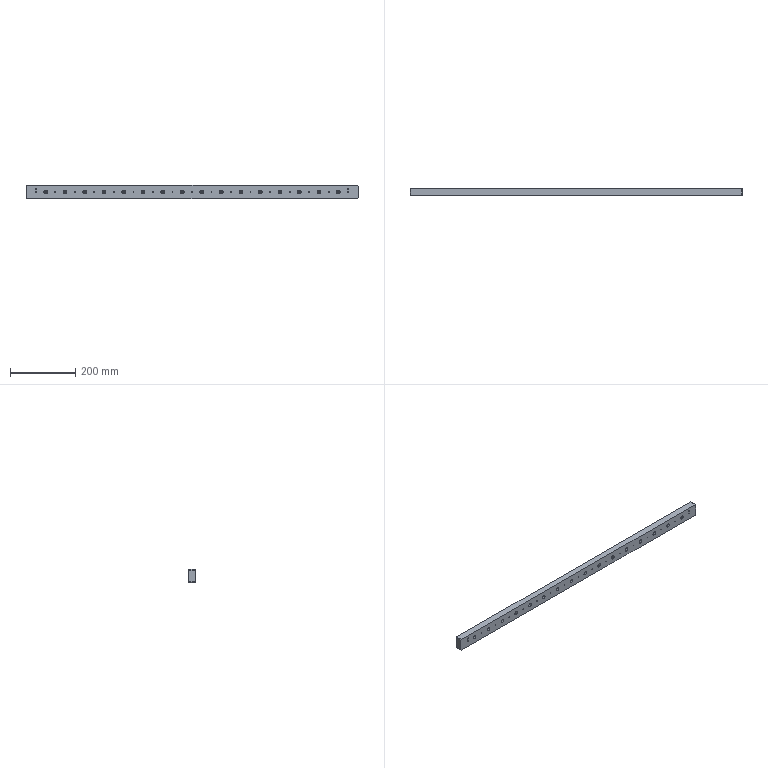Part | SolidWorks | features HoleWzd 3, LPattern 2, Chamfer 1, Extrusion 1 | 1 solid | 166 faces | box 1020 x 20 x 40 mm | volume 797316 mm3 | cylinder 102 | cone 38 | plane 26 | commonest cylinder face diameters 2.5 x34 6.6 x32 11 x32 4 x4